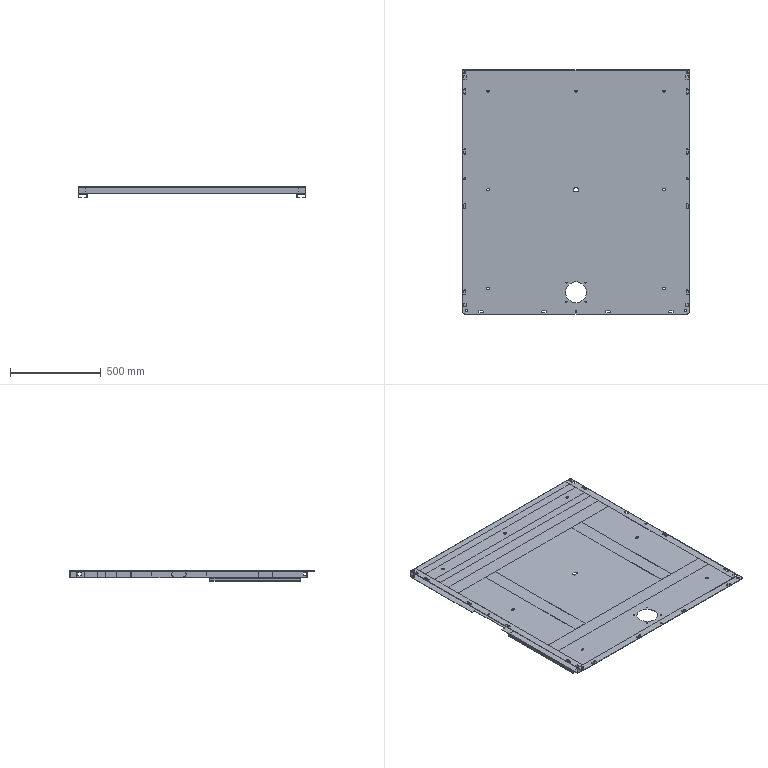Part | SolidWorks | features ReferencePattern 5, MirrorCompFeat 4, LocalLPattern 1 | 19 solids | 1142 faces | box 1250 x 1345 x 59.5 mm | volume 5102202 mm3 | plane 774 | cylinder 344 | cone 24 | commonest cylinder face diameters 10 x84 0.4 x50 3.4 x48 20 x39 11 x37 30 x10